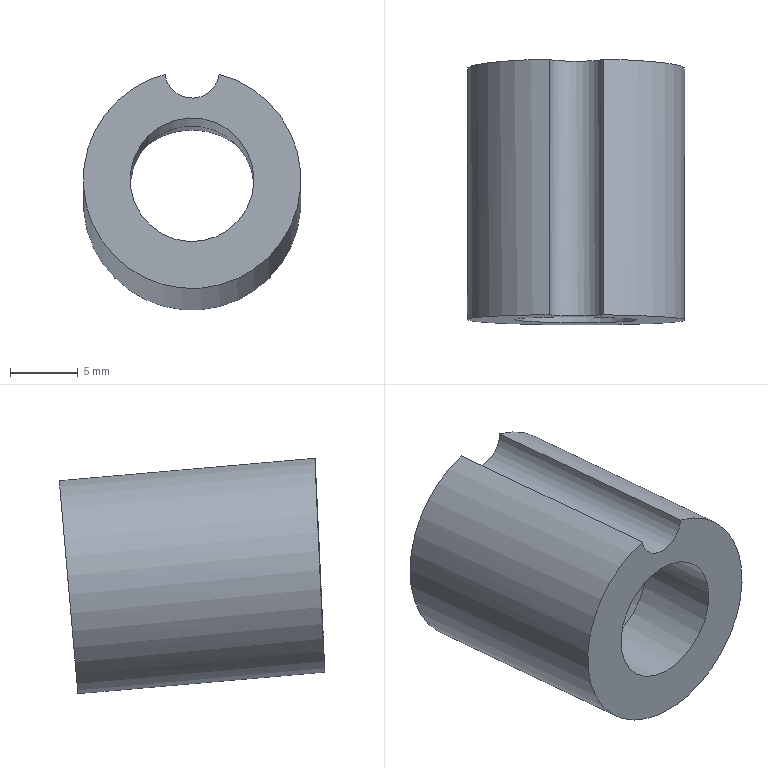Part | NX | features EKSD 16-20-9.100 2 | 1 solid | 7 faces | box 16 x 19.518 x 17.335 mm | volume 2132 mm3 | cylinder 4 | plane 3 | commonest cylinder face diameters 4 x1 9.1 x1 10.6 x1 16 x1
STEP:
#1=CARTESIAN_POINT('',(154.539,-27.697,-43.269));
#2=VERTEX_POINT('',#1);
#3=CARTESIAN_POINT('',(158.508,-27.697,-43.269));
#4=VERTEX_POINT('',#3);
#5=CARTESIAN_POINT('',(156.524,-27.675,-43.02));
#6=DIRECTION('',(0.,-0.9962,0.08716));
#7=DIRECTION('',(0.,-0.08716,-0.9962));
#8=AXIS2_PLACEMENT_3D('',#5,#6,#7);
#9=CIRCLE('',#8,2.);
#10=EDGE_CURVE('',#2,#4,#9,.T.);
#11=ORIENTED_EDGE('',*,*,#10,.T.);
#12=CARTESIAN_POINT('',(156.524,-28.372,-50.99));
#13=DIRECTION('',(0.,-0.9962,0.08716));
#14=DIRECTION('',(0.,-0.08716,-0.9962));
#15=AXIS2_PLACEMENT_3D('',#12,#13,#14);
#16=CIRCLE('',#15,8.);
#17=EDGE_CURVE('',#2,#4,#16,.T.);
#18=ORIENTED_EDGE('',*,*,#17,.F.);
#19=EDGE_LOOP('',(#11,#18));
#20=FACE_BOUND('',#19,.T.);
#21=CARTESIAN_POINT('',(156.524,-27.91,-45.71));
#22=VERTEX_POINT('',#21);
#23=CARTESIAN_POINT('',(156.524,-28.372,-50.99));
#24=DIRECTION('',(0.,0.9962,-0.08716));
#25=DIRECTION('',(0.,0.08716,0.9962));
#26=AXIS2_PLACEMENT_3D('',#23,#24,#25);
#27=CIRCLE('',#26,5.3);
#28=EDGE_CURVE('',#22,#22,#27,.T.);
#29=ORIENTED_EDGE('',*,*,#28,.F.);
#30=EDGE_LOOP('',(#29));
#31=FACE_BOUND('',#30,.T.);
#32=CARTESIAN_POINT('',(156.524,-28.372,-50.99));
#33=DIRECTION('',(0.,0.9962,-0.08716));
#34=DIRECTION('',(0.,0.08716,0.9962));
#35=AXIS2_PLACEMENT_3D('',#32,#33,#34);
#36=PLANE('',#35);
#37=ADVANCED_FACE('',(#20,#31),#36,.T.);
#38=CARTESIAN_POINT('',(158.508,-46.502,-41.624));
#39=VERTEX_POINT('',#38);
#40=CARTESIAN_POINT('',(154.539,-46.494,-41.625));
#41=VERTEX_POINT('',#40);
#42=CARTESIAN_POINT('',(156.524,-46.487,-41.374));
#43=DIRECTION('',(0.001957,0.999,-0.04546));
#44=DIRECTION('',(-0.04675,-0.04532,-0.9979));
#45=AXIS2_PLACEMENT_3D('',#42,#43,#44);
#46=ELLIPSE('',#45,2.002,2.);
#47=EDGE_CURVE('',#39,#41,#46,.T.);
#48=ORIENTED_EDGE('',*,*,#47,.T.);
#49=CARTESIAN_POINT('',(156.524,-46.851,-49.373));
#50=DIRECTION('',(0.001957,0.999,-0.04546));
#51=DIRECTION('',(-0.04675,-0.04532,-0.9979));
#52=AXIS2_PLACEMENT_3D('',#49,#50,#51);
#53=ELLIPSE('',#52,8.007,8.);
#54=EDGE_CURVE('',#39,#41,#53,.T.);
#55=ORIENTED_EDGE('',*,*,#54,.F.);
#56=EDGE_LOOP('',(#48,#55));
#57=FACE_BOUND('',#56,.T.);
#58=CARTESIAN_POINT('',(156.311,-47.057,-53.917));
#59=VERTEX_POINT('',#58);
#60=CARTESIAN_POINT('',(156.524,-46.851,-49.373));
#61=DIRECTION('',(0.001957,0.999,-0.04546));
#62=DIRECTION('',(-0.04675,-0.04532,-0.9979));
#63=AXIS2_PLACEMENT_3D('',#60,#61,#62);
#64=ELLIPSE('',#63,4.554,4.55);
#65=EDGE_CURVE('',#59,#59,#64,.F.);
#66=ORIENTED_EDGE('',*,*,#65,.F.);
#67=EDGE_LOOP('',(#66));
#68=FACE_BOUND('',#67,.T.);
#69=CARTESIAN_POINT('',(128.811,-48.589,-88.763));
#70=DIRECTION('',(0.001957,0.999,-0.04546));
#71=DIRECTION('',(0.06617,0.04523,0.9968));
#72=AXIS2_PLACEMENT_3D('',#69,#70,#71);
#73=PLANE('',#72);
#74=ADVANCED_FACE('',(#57,#68),#73,.F.);
#75=CARTESIAN_POINT('',(158.508,-37.659,-42.398));
#76=DIRECTION('',(0.,0.9962,-0.08716));
#77=VECTOR('',#76,1000.);
#78=LINE('',#75,#77);
#79=EDGE_CURVE('',#39,#4,#78,.T.);
#80=ORIENTED_EDGE('',*,*,#79,.F.);
#81=ORIENTED_EDGE('',*,*,#54,.T.);
#82=CARTESIAN_POINT('',(154.539,-37.659,-42.398));
#83=DIRECTION('',(0.,0.9962,-0.08716));
#84=VECTOR('',#83,1000.);
#85=LINE('',#82,#84);
#86=EDGE_CURVE('',#2,#41,#85,.F.);
#87=ORIENTED_EDGE('',*,*,#86,.F.);
#88=ORIENTED_EDGE('',*,*,#17,.T.);
#89=EDGE_LOOP('',(#80,#81,#87,#88));
#90=FACE_BOUND('',#89,.T.);
#91=CARTESIAN_POINT('',(156.524,-48.296,-49.247));
#92=DIRECTION('',(0.,0.9962,-0.08716));
#93=DIRECTION('',(0.,0.08716,0.9962));
#94=AXIS2_PLACEMENT_3D('',#91,#92,#93);
#95=CYLINDRICAL_SURFACE('',#94,8.);
#96=ADVANCED_FACE('',(#90),#95,.T.);
#97=CARTESIAN_POINT('',(156.524,-40.723,-54.477));
#98=VERTEX_POINT('',#97);
#99=CARTESIAN_POINT('',(156.524,-40.327,-49.944));
#100=DIRECTION('',(0.,-0.9962,0.08716));
#101=DIRECTION('',(0.,-0.08716,-0.9962));
#102=AXIS2_PLACEMENT_3D('',#99,#100,#101);
#103=CIRCLE('',#102,4.55);
#104=EDGE_CURVE('',#98,#98,#103,.F.);
#105=ORIENTED_EDGE('',*,*,#104,.T.);
#106=EDGE_LOOP('',(#105));
#107=FACE_BOUND('',#106,.T.);
#108=ORIENTED_EDGE('',*,*,#65,.T.);
#109=EDGE_LOOP('',(#108));
#110=FACE_BOUND('',#109,.T.);
#111=CARTESIAN_POINT('',(156.524,-49.292,-49.159));
#112=DIRECTION('',(0.,0.9962,-0.08716));
#113=DIRECTION('',(0.,0.08716,0.9962));
#114=AXIS2_PLACEMENT_3D('',#111,#112,#113);
#115=CYLINDRICAL_SURFACE('',#114,4.55);
#116=ADVANCED_FACE('',(#107,#110),#115,.F.);
#117=CARTESIAN_POINT('',(156.524,-39.865,-44.664));
#118=VERTEX_POINT('',#117);
#119=CARTESIAN_POINT('',(156.524,-40.327,-49.944));
#120=DIRECTION('',(0.,0.9962,-0.08716));
#121=DIRECTION('',(0.,0.08716,0.9962));
#122=AXIS2_PLACEMENT_3D('',#119,#120,#121);
#123=CIRCLE('',#122,5.3);
#124=EDGE_CURVE('',#118,#118,#123,.T.);
#125=ORIENTED_EDGE('',*,*,#124,.T.);
#126=EDGE_LOOP('',(#125));
#127=FACE_BOUND('',#126,.T.);
#128=ORIENTED_EDGE('',*,*,#104,.F.);
#129=EDGE_LOOP('',(#128));
#130=FACE_BOUND('',#129,.T.);
#131=CARTESIAN_POINT('',(156.524,-40.327,-49.944));
#132=DIRECTION('',(0.,-0.9962,0.08716));
#133=DIRECTION('',(0.,-0.08716,-0.9962));
#134=AXIS2_PLACEMENT_3D('',#131,#132,#133);
#135=PLANE('',#134);
#136=ADVANCED_FACE('',(#127,#130),#135,.F.);
#137=ORIENTED_EDGE('',*,*,#28,.T.);
#138=EDGE_LOOP('',(#137));
#139=FACE_BOUND('',#138,.T.);
#140=ORIENTED_EDGE('',*,*,#124,.F.);
#141=EDGE_LOOP('',(#140));
#142=FACE_BOUND('',#141,.T.);
#143=CARTESIAN_POINT('',(156.524,-40.327,-49.944));
#144=DIRECTION('',(0.,0.9962,-0.08716));
#145=DIRECTION('',(0.,0.08716,0.9962));
#146=AXIS2_PLACEMENT_3D('',#143,#144,#145);
#147=CYLINDRICAL_SURFACE('',#146,5.3);
#148=ADVANCED_FACE('',(#139,#142),#147,.F.);
#149=ORIENTED_EDGE('',*,*,#79,.T.);
#150=ORIENTED_EDGE('',*,*,#10,.F.);
#151=ORIENTED_EDGE('',*,*,#86,.T.);
#152=ORIENTED_EDGE('',*,*,#47,.F.);
#153=EDGE_LOOP('',(#149,#150,#151,#152));
#154=FACE_BOUND('',#153,.T.);
#155=CARTESIAN_POINT('',(156.524,-47.599,-41.277));
#156=DIRECTION('',(0.,0.9962,-0.08716));
#157=DIRECTION('',(0.,0.08716,0.9962));
#158=AXIS2_PLACEMENT_3D('',#155,#156,#157);
#159=CYLINDRICAL_SURFACE('',#158,2.);
#160=ADVANCED_FACE('',(#154),#159,.F.);
#161=CLOSED_SHELL('',(#37,#74,#96,#116,#136,#148,#160));
#162=MANIFOLD_SOLID_BREP('',#161);
#163=(LENGTH_UNIT()NAMED_UNIT(*)SI_UNIT(.MILLI.,.METRE.));
#164=UNCERTAINTY_MEASURE_WITH_UNIT(LENGTH_MEASURE(0.00001),#163,'','');
#165=(NAMED_UNIT(*)PLANE_ANGLE_UNIT()SI_UNIT($,.RADIAN.));
#166=(NAMED_UNIT(*)SI_UNIT($,.STERADIAN.)SOLID_ANGLE_UNIT());
#167=(GEOMETRIC_REPRESENTATION_CONTEXT(3)GLOBAL_UNCERTAINTY_ASSIGNED_CONTEXT((#164))GLOBAL_UNIT_ASSIGNED_CONTEXT((#163,#165,#166))REPRESENTATION_CONTEXT('',''));
#168=ADVANCED_BREP_SHAPE_REPRESENTATION('',(#162),#167);